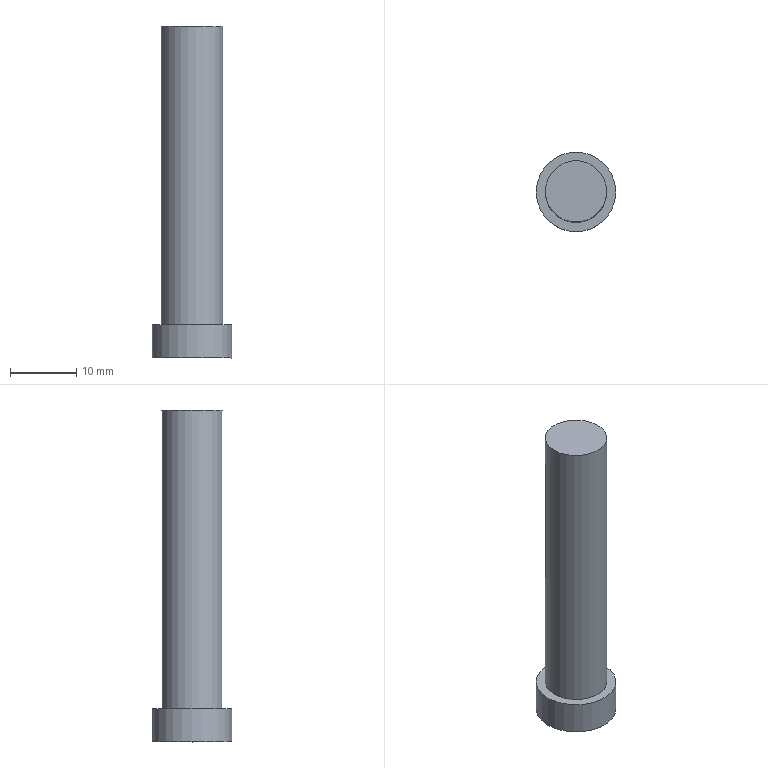Part | NX | features solid 2 | 1 solid | 5 faces | box 12 x 12 x 50 mm | volume 3590 mm3 | plane 3 | cylinder 2 | commonest cylinder face diameters 9.25 x1 12 x1
STEP:
#1=CARTESIAN_POINT('',(3117.891,-809.538,862.716));
#2=VERTEX_POINT('',#1);
#3=CARTESIAN_POINT('',(3113.266,-809.538,862.716));
#4=DIRECTION('',(0.,0.,1.));
#5=DIRECTION('',(1.,0.,0.));
#6=AXIS2_PLACEMENT_3D('',#3,#4,#5);
#7=CIRCLE('',#6,4.625);
#8=EDGE_CURVE('',#2,#2,#7,.F.);
#9=ORIENTED_EDGE('',*,*,#8,.F.);
#10=EDGE_LOOP('',(#9));
#11=FACE_BOUND('',#10,.T.);
#12=CARTESIAN_POINT('',(3113.266,-809.538,862.716));
#13=DIRECTION('',(0.,0.,1.));
#14=DIRECTION('',(1.,0.,0.));
#15=AXIS2_PLACEMENT_3D('',#12,#13,#14);
#16=PLANE('',#15);
#17=ADVANCED_FACE('',(#11),#16,.T.);
#18=ORIENTED_EDGE('',*,*,#8,.T.);
#19=EDGE_LOOP('',(#18));
#20=FACE_BOUND('',#19,.T.);
#21=CARTESIAN_POINT('',(3108.641,-809.538,817.716));
#22=VERTEX_POINT('',#21);
#23=CARTESIAN_POINT('',(3113.266,-809.538,817.716));
#24=DIRECTION('',(0.,0.,-1.));
#25=DIRECTION('',(-1.,0.,0.));
#26=AXIS2_PLACEMENT_3D('',#23,#24,#25);
#27=CIRCLE('',#26,4.625);
#28=EDGE_CURVE('',#22,#22,#27,.T.);
#29=ORIENTED_EDGE('',*,*,#28,.F.);
#30=EDGE_LOOP('',(#29));
#31=FACE_BOUND('',#30,.T.);
#32=CARTESIAN_POINT('',(3113.266,-809.538,862.716));
#33=DIRECTION('',(0.,0.,-1.));
#34=DIRECTION('',(-1.,0.,0.));
#35=AXIS2_PLACEMENT_3D('',#32,#33,#34);
#36=CYLINDRICAL_SURFACE('',#35,4.625);
#37=ADVANCED_FACE('',(#20,#31),#36,.T.);
#38=CARTESIAN_POINT('',(3107.266,-809.538,817.716));
#39=VERTEX_POINT('',#38);
#40=CARTESIAN_POINT('',(3113.266,-809.538,817.716));
#41=DIRECTION('',(0.,0.,-1.));
#42=DIRECTION('',(-1.,0.,0.));
#43=AXIS2_PLACEMENT_3D('',#40,#41,#42);
#44=CIRCLE('',#43,6.);
#45=EDGE_CURVE('',#39,#39,#44,.F.);
#46=ORIENTED_EDGE('',*,*,#45,.F.);
#47=EDGE_LOOP('',(#46));
#48=FACE_BOUND('',#47,.T.);
#49=CARTESIAN_POINT('',(3107.266,-809.538,812.716));
#50=VERTEX_POINT('',#49);
#51=CARTESIAN_POINT('',(3113.266,-809.538,812.716));
#52=DIRECTION('',(0.,0.,-1.));
#53=DIRECTION('',(-1.,0.,0.));
#54=AXIS2_PLACEMENT_3D('',#51,#52,#53);
#55=CIRCLE('',#54,6.);
#56=EDGE_CURVE('',#50,#50,#55,.T.);
#57=ORIENTED_EDGE('',*,*,#56,.F.);
#58=EDGE_LOOP('',(#57));
#59=FACE_BOUND('',#58,.T.);
#60=CARTESIAN_POINT('',(3113.266,-809.538,851.716));
#61=DIRECTION('',(0.,0.,-1.));
#62=DIRECTION('',(-1.,0.,0.));
#63=AXIS2_PLACEMENT_3D('',#60,#61,#62);
#64=CYLINDRICAL_SURFACE('',#63,6.);
#65=ADVANCED_FACE('',(#48,#59),#64,.T.);
#66=ORIENTED_EDGE('',*,*,#56,.T.);
#67=EDGE_LOOP('',(#66));
#68=FACE_BOUND('',#67,.T.);
#69=CARTESIAN_POINT('',(3113.266,-809.538,812.716));
#70=DIRECTION('',(0.,0.,-1.));
#71=DIRECTION('',(0.0349,-0.9994,0.));
#72=AXIS2_PLACEMENT_3D('',#69,#70,#71);
#73=PLANE('',#72);
#74=ADVANCED_FACE('',(#68),#73,.T.);
#75=ORIENTED_EDGE('',*,*,#28,.T.);
#76=EDGE_LOOP('',(#75));
#77=FACE_BOUND('',#76,.T.);
#78=ORIENTED_EDGE('',*,*,#45,.T.);
#79=EDGE_LOOP('',(#78));
#80=FACE_BOUND('',#79,.T.);
#81=CARTESIAN_POINT('',(3113.266,-809.538,817.716));
#82=DIRECTION('',(0.,0.,-1.));
#83=DIRECTION('',(-1.,0.,0.));
#84=AXIS2_PLACEMENT_3D('',#81,#82,#83);
#85=PLANE('',#84);
#86=ADVANCED_FACE('',(#77,#80),#85,.F.);
#87=CLOSED_SHELL('',(#17,#37,#65,#74,#86));
#88=MANIFOLD_SOLID_BREP('',#87);
#89=(LENGTH_UNIT()NAMED_UNIT(*)SI_UNIT(.MILLI.,.METRE.));
#90=UNCERTAINTY_MEASURE_WITH_UNIT(LENGTH_MEASURE(0.00001),#89,'','');
#91=(NAMED_UNIT(*)PLANE_ANGLE_UNIT()SI_UNIT($,.RADIAN.));
#92=(NAMED_UNIT(*)SI_UNIT($,.STERADIAN.)SOLID_ANGLE_UNIT());
#93=(GEOMETRIC_REPRESENTATION_CONTEXT(3)GLOBAL_UNCERTAINTY_ASSIGNED_CONTEXT((#90))GLOBAL_UNIT_ASSIGNED_CONTEXT((#89,#91,#92))REPRESENTATION_CONTEXT('',''));
#94=ADVANCED_BREP_SHAPE_REPRESENTATION('',(#88),#93);